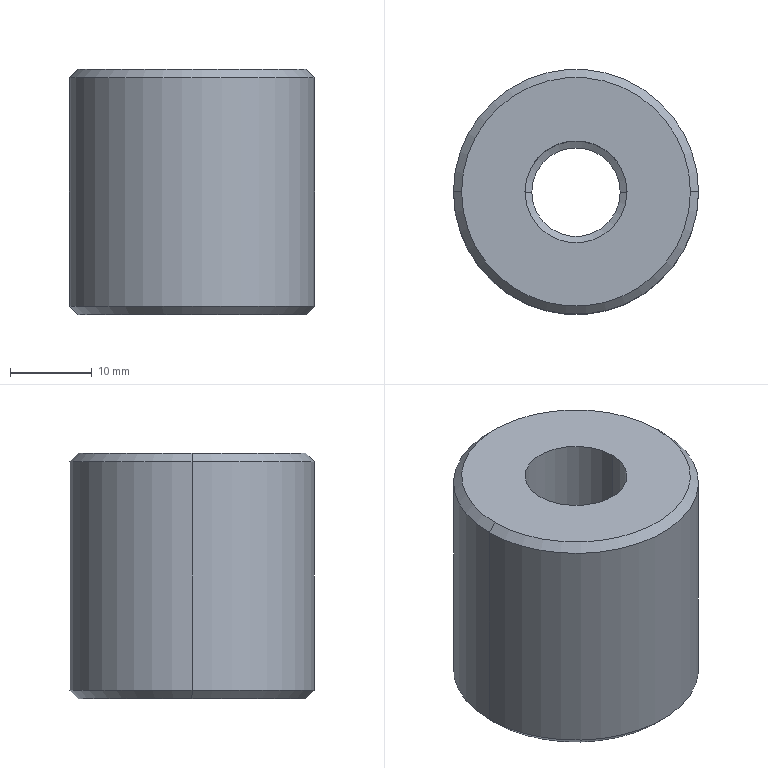Part | STEP file | Locking Cylinder Joint | 1 solid | 15 faces | box 30 x 30 x 30 mm | volume 16100 mm3 | cone 6 | cylinder 6 | plane 3 | commonest cylinder face diameters 12.5 x2 20 x2 30 x2
STEP:
#1=CARTESIAN_POINT('',(0.,0.,0.));
#2=DIRECTION('',(0.,0.,1.));
#3=DIRECTION('',(1.,0.,0.));
#4=AXIS2_PLACEMENT_3D('',#1,#2,#3);
#5=CARTESIAN_POINT('',(-14.,0.,0.));
#6=VERTEX_POINT('',#5);
#7=CARTESIAN_POINT('',(14.,0.,0.));
#8=VERTEX_POINT('',#7);
#9=CARTESIAN_POINT('',(0.,0.,0.));
#10=DIRECTION('',(0.,0.,-1.));
#11=DIRECTION('',(1.,0.,0.));
#12=AXIS2_PLACEMENT_3D('',#9,#10,#11);
#13=CIRCLE('',#12,14.);
#14=CARTESIAN_POINT('',(0.,0.,1.));
#15=DIRECTION('',(0.,0.,1.));
#16=DIRECTION('',(1.,0.,0.));
#17=AXIS2_PLACEMENT_3D('',#14,#15,#16);
#18=CONICAL_SURFACE('',#17,15.,0.7854);
#19=CARTESIAN_POINT('',(6.283,-1.));
#20=DIRECTION('',(-1.,0.));
#21=VECTOR('',#20,1.);
#22=LINE('',#19,#21);
#23=(GEOMETRIC_REPRESENTATION_CONTEXT(2)PARAMETRIC_REPRESENTATION_CONTEXT()REPRESENTATION_CONTEXT('',''));
#24=DEFINITIONAL_REPRESENTATION('',(#22),#23);
#25=PCURVE('',#18,#24);
#26=CARTESIAN_POINT('',(0.,0.,0.));
#27=DIRECTION('',(0.,0.,1.));
#28=DIRECTION('',(1.,0.,0.));
#29=AXIS2_PLACEMENT_3D('',#26,#27,#28);
#30=PLANE('',#29);
#31=CARTESIAN_POINT('',(14.,0.));
#32=CARTESIAN_POINT('',(14.,-24.249));
#33=CARTESIAN_POINT('',(-7.,-12.124));
#34=CARTESIAN_POINT('',(-28.,0.));
#35=CARTESIAN_POINT('',(-7.,12.124));
#36=CARTESIAN_POINT('',(14.,24.249));
#37=CARTESIAN_POINT('',(14.,0.));
#38=(BOUNDED_CURVE()B_SPLINE_CURVE(2,(#31,#32,#33,#34,#35,#36,#37),.UNSPECIFIED.,.T.,.F.)B_SPLINE_CURVE_WITH_KNOTS((1,2,2,2,2,1),(-2.094,0.,2.094,4.189,6.283,8.378),.UNSPECIFIED.)CURVE()GEOMETRIC_REPRESENTATION_ITEM()RATIONAL_B_SPLINE_CURVE((1.,0.5,1.,0.5,1.,0.5,1.))REPRESENTATION_ITEM(''));
#39=(GEOMETRIC_REPRESENTATION_CONTEXT(2)PARAMETRIC_REPRESENTATION_CONTEXT()REPRESENTATION_CONTEXT('',''));
#40=DEFINITIONAL_REPRESENTATION('',(#38),#39);
#41=PCURVE('',#30,#40);
#42=SURFACE_CURVE('',#13,(#25,#41),.PCURVE_S1.);
#43=EDGE_CURVE('',#6,#8,#42,.T.);
#44=ORIENTED_EDGE('',*,*,#43,.F.);
#45=CARTESIAN_POINT('',(-15.,0.,1.));
#46=VERTEX_POINT('',#45);
#47=CARTESIAN_POINT('',(-15.,0.,1.));
#48=DIRECTION('',(-0.7071,0.,0.7071));
#49=VECTOR('',#48,1.);
#50=LINE('',#47,#49);
#51=CARTESIAN_POINT('',(3.142,0.));
#52=DIRECTION('',(0.,1.));
#53=VECTOR('',#52,1.);
#54=LINE('',#51,#53);
#55=(GEOMETRIC_REPRESENTATION_CONTEXT(2)PARAMETRIC_REPRESENTATION_CONTEXT()REPRESENTATION_CONTEXT('',''));
#56=DEFINITIONAL_REPRESENTATION('',(#54),#55);
#57=PCURVE('',#18,#56);
#58=CARTESIAN_POINT('',(0.,0.,1.));
#59=DIRECTION('',(0.,0.,1.));
#60=DIRECTION('',(1.,0.,0.));
#61=AXIS2_PLACEMENT_3D('',#58,#59,#60);
#62=CONICAL_SURFACE('',#61,15.,0.7854);
#63=CARTESIAN_POINT('',(3.142,0.));
#64=DIRECTION('',(0.,1.));
#65=VECTOR('',#64,1.);
#66=LINE('',#63,#65);
#67=(GEOMETRIC_REPRESENTATION_CONTEXT(2)PARAMETRIC_REPRESENTATION_CONTEXT()REPRESENTATION_CONTEXT('',''));
#68=DEFINITIONAL_REPRESENTATION('',(#66),#67);
#69=PCURVE('',#62,#68);
#70=SURFACE_CURVE('',#50,(#57,#69),.PCURVE_S1.);
#71=EDGE_CURVE('',#6,#46,#70,.T.);
#72=ORIENTED_EDGE('',*,*,#71,.T.);
#73=CARTESIAN_POINT('',(15.,0.,1.));
#74=VERTEX_POINT('',#73);
#75=CARTESIAN_POINT('',(0.,0.,1.));
#76=DIRECTION('',(0.,0.,1.));
#77=DIRECTION('',(1.,0.,0.));
#78=AXIS2_PLACEMENT_3D('',#75,#76,#77);
#79=CIRCLE('',#78,15.);
#80=CARTESIAN_POINT('',(0.,0.));
#81=DIRECTION('',(1.,0.));
#82=VECTOR('',#81,1.);
#83=LINE('',#80,#82);
#84=(GEOMETRIC_REPRESENTATION_CONTEXT(2)PARAMETRIC_REPRESENTATION_CONTEXT()REPRESENTATION_CONTEXT('',''));
#85=DEFINITIONAL_REPRESENTATION('',(#83),#84);
#86=PCURVE('',#18,#85);
#87=CARTESIAN_POINT('',(0.,0.,30.));
#88=DIRECTION('',(0.,0.,-1.));
#89=DIRECTION('',(-1.,0.,0.));
#90=AXIS2_PLACEMENT_3D('',#87,#88,#89);
#91=CYLINDRICAL_SURFACE('',#90,15.);
#92=CARTESIAN_POINT('',(3.142,29.));
#93=DIRECTION('',(-1.,0.));
#94=VECTOR('',#93,1.);
#95=LINE('',#92,#94);
#96=(GEOMETRIC_REPRESENTATION_CONTEXT(2)PARAMETRIC_REPRESENTATION_CONTEXT()REPRESENTATION_CONTEXT('',''));
#97=DEFINITIONAL_REPRESENTATION('',(#95),#96);
#98=PCURVE('',#91,#97);
#99=SURFACE_CURVE('',#79,(#86,#98),.PCURVE_S1.);
#100=EDGE_CURVE('',#74,#46,#99,.T.);
#101=ORIENTED_EDGE('',*,*,#100,.F.);
#102=CARTESIAN_POINT('',(15.,0.,1.));
#103=DIRECTION('',(0.7071,0.,0.7071));
#104=VECTOR('',#103,1.);
#105=LINE('',#102,#104);
#106=CARTESIAN_POINT('',(0.,0.));
#107=DIRECTION('',(0.,1.));
#108=VECTOR('',#107,1.);
#109=LINE('',#106,#108);
#110=(GEOMETRIC_REPRESENTATION_CONTEXT(2)PARAMETRIC_REPRESENTATION_CONTEXT()REPRESENTATION_CONTEXT('',''));
#111=DEFINITIONAL_REPRESENTATION('',(#109),#110);
#112=PCURVE('',#18,#111);
#113=CARTESIAN_POINT('',(6.283,0.));
#114=DIRECTION('',(0.,1.));
#115=VECTOR('',#114,1.);
#116=LINE('',#113,#115);
#117=(GEOMETRIC_REPRESENTATION_CONTEXT(2)PARAMETRIC_REPRESENTATION_CONTEXT()REPRESENTATION_CONTEXT('',''));
#118=DEFINITIONAL_REPRESENTATION('',(#116),#117);
#119=PCURVE('',#62,#118);
#120=SURFACE_CURVE('',#105,(#112,#119),.PCURVE_S1.);
#121=EDGE_CURVE('',#8,#74,#120,.T.);
#122=ORIENTED_EDGE('',*,*,#121,.F.);
#123=EDGE_LOOP('',(#44,#72,#101,#122));
#124=FACE_BOUND('',#123,.T.);
#125=ADVANCED_FACE('',(#124),#18,.T.);
#126=CARTESIAN_POINT('',(14.,0.,30.));
#127=VERTEX_POINT('',#126);
#128=CARTESIAN_POINT('',(-14.,0.,30.));
#129=VERTEX_POINT('',#128);
#130=CARTESIAN_POINT('',(0.,0.,30.));
#131=DIRECTION('',(0.,0.,1.));
#132=DIRECTION('',(1.,0.,0.));
#133=AXIS2_PLACEMENT_3D('',#130,#131,#132);
#134=CIRCLE('',#133,14.);
#135=CARTESIAN_POINT('',(0.,0.,30.));
#136=DIRECTION('',(0.,0.,-1.));
#137=DIRECTION('',(-1.,0.,0.));
#138=AXIS2_PLACEMENT_3D('',#135,#136,#137);
#139=CONICAL_SURFACE('',#138,14.,0.7854);
#140=CARTESIAN_POINT('',(3.142,0.));
#141=DIRECTION('',(-1.,0.));
#142=VECTOR('',#141,1.);
#143=LINE('',#140,#142);
#144=(GEOMETRIC_REPRESENTATION_CONTEXT(2)PARAMETRIC_REPRESENTATION_CONTEXT()REPRESENTATION_CONTEXT('',''));
#145=DEFINITIONAL_REPRESENTATION('',(#143),#144);
#146=PCURVE('',#139,#145);
#147=CARTESIAN_POINT('',(0.,0.,30.));
#148=DIRECTION('',(0.,0.,1.));
#149=DIRECTION('',(1.,0.,0.));
#150=AXIS2_PLACEMENT_3D('',#147,#148,#149);
#151=PLANE('',#150);
#152=CARTESIAN_POINT('',(0.,0.));
#153=DIRECTION('',(1.,0.));
#154=AXIS2_PLACEMENT_2D('',#152,#153);
#155=CIRCLE('',#154,14.);
#156=(GEOMETRIC_REPRESENTATION_CONTEXT(2)PARAMETRIC_REPRESENTATION_CONTEXT()REPRESENTATION_CONTEXT('',''));
#157=DEFINITIONAL_REPRESENTATION('',(#155),#156);
#158=PCURVE('',#151,#157);
#159=SURFACE_CURVE('',#134,(#146,#158),.PCURVE_S1.);
#160=EDGE_CURVE('',#127,#129,#159,.T.);
#161=ORIENTED_EDGE('',*,*,#160,.F.);
#162=CARTESIAN_POINT('',(15.,0.,29.));
#163=VERTEX_POINT('',#162);
#164=CARTESIAN_POINT('',(14.,0.,30.));
#165=DIRECTION('',(0.7071,0.,-0.7071));
#166=VECTOR('',#165,1.);
#167=LINE('',#164,#166);
#168=CARTESIAN_POINT('',(3.142,0.));
#169=DIRECTION('',(0.,1.));
#170=VECTOR('',#169,1.);
#171=LINE('',#168,#170);
#172=(GEOMETRIC_REPRESENTATION_CONTEXT(2)PARAMETRIC_REPRESENTATION_CONTEXT()REPRESENTATION_CONTEXT('',''));
#173=DEFINITIONAL_REPRESENTATION('',(#171),#172);
#174=PCURVE('',#139,#173);
#175=CARTESIAN_POINT('',(0.,0.,30.));
#176=DIRECTION('',(0.,0.,-1.));
#177=DIRECTION('',(-1.,0.,0.));
#178=AXIS2_PLACEMENT_3D('',#175,#176,#177);
#179=CONICAL_SURFACE('',#178,14.,0.7854);
#180=CARTESIAN_POINT('',(3.142,0.));
#181=DIRECTION('',(0.,1.));
#182=VECTOR('',#181,1.);
#183=LINE('',#180,#182);
#184=(GEOMETRIC_REPRESENTATION_CONTEXT(2)PARAMETRIC_REPRESENTATION_CONTEXT()REPRESENTATION_CONTEXT('',''));
#185=DEFINITIONAL_REPRESENTATION('',(#183),#184);
#186=PCURVE('',#179,#185);
#187=SURFACE_CURVE('',#167,(#174,#186),.PCURVE_S1.);
#188=EDGE_CURVE('',#127,#163,#187,.T.);
#189=ORIENTED_EDGE('',*,*,#188,.T.);
#190=CARTESIAN_POINT('',(-15.,0.,29.));
#191=VERTEX_POINT('',#190);
#192=CARTESIAN_POINT('',(0.,0.,29.));
#193=DIRECTION('',(0.,0.,-1.));
#194=DIRECTION('',(1.,0.,0.));
#195=AXIS2_PLACEMENT_3D('',#192,#193,#194);
#196=CIRCLE('',#195,15.);
#197=CARTESIAN_POINT('',(-3.142,1.));
#198=DIRECTION('',(1.,0.));
#199=VECTOR('',#198,1.);
#200=LINE('',#197,#199);
#201=(GEOMETRIC_REPRESENTATION_CONTEXT(2)PARAMETRIC_REPRESENTATION_CONTEXT()REPRESENTATION_CONTEXT('',''));
#202=DEFINITIONAL_REPRESENTATION('',(#200),#201);
#203=PCURVE('',#139,#202);
#204=CARTESIAN_POINT('',(-3.142,1.));
#205=DIRECTION('',(1.,0.));
#206=VECTOR('',#205,1.);
#207=LINE('',#204,#206);
#208=(GEOMETRIC_REPRESENTATION_CONTEXT(2)PARAMETRIC_REPRESENTATION_CONTEXT()REPRESENTATION_CONTEXT('',''));
#209=DEFINITIONAL_REPRESENTATION('',(#207),#208);
#210=PCURVE('',#91,#209);
#211=SURFACE_CURVE('',#196,(#203,#210),.PCURVE_S1.);
#212=EDGE_CURVE('',#191,#163,#211,.T.);
#213=ORIENTED_EDGE('',*,*,#212,.F.);
#214=CARTESIAN_POINT('',(-14.,0.,30.));
#215=DIRECTION('',(-0.7071,0.,-0.7071));
#216=VECTOR('',#215,1.);
#217=LINE('',#214,#216);
#218=CARTESIAN_POINT('',(0.,0.));
#219=DIRECTION('',(0.,1.));
#220=VECTOR('',#219,1.);
#221=LINE('',#218,#220);
#222=(GEOMETRIC_REPRESENTATION_CONTEXT(2)PARAMETRIC_REPRESENTATION_CONTEXT()REPRESENTATION_CONTEXT('',''));
#223=DEFINITIONAL_REPRESENTATION('',(#221),#222);
#224=PCURVE('',#139,#223);
#225=CARTESIAN_POINT('',(6.283,0.));
#226=DIRECTION('',(0.,1.));
#227=VECTOR('',#226,1.);
#228=LINE('',#225,#227);
#229=(GEOMETRIC_REPRESENTATION_CONTEXT(2)PARAMETRIC_REPRESENTATION_CONTEXT()REPRESENTATION_CONTEXT('',''));
#230=DEFINITIONAL_REPRESENTATION('',(#228),#229);
#231=PCURVE('',#179,#230);
#232=SURFACE_CURVE('',#217,(#224,#231),.PCURVE_S1.);
#233=EDGE_CURVE('',#129,#191,#232,.T.);
#234=ORIENTED_EDGE('',*,*,#233,.F.);
#235=EDGE_LOOP('',(#161,#189,#213,#234));
#236=FACE_BOUND('',#235,.T.);
#237=ADVANCED_FACE('',(#236),#139,.T.);
#238=CARTESIAN_POINT('',(-10.,0.,7.));
#239=VERTEX_POINT('',#238);
#240=CARTESIAN_POINT('',(-10.,0.,0.));
#241=VERTEX_POINT('',#240);
#242=CARTESIAN_POINT('',(-10.,0.,7.));
#243=DIRECTION('',(0.,0.,-1.));
#244=VECTOR('',#243,1.);
#245=LINE('',#242,#244);
#246=CARTESIAN_POINT('',(0.,0.,7.));
#247=DIRECTION('',(0.,0.,-1.));
#248=DIRECTION('',(-1.,0.,0.));
#249=AXIS2_PLACEMENT_3D('',#246,#247,#248);
#250=CYLINDRICAL_SURFACE('',#249,10.);
#251=CARTESIAN_POINT('',(6.283,0.));
#252=DIRECTION('',(0.,1.));
#253=VECTOR('',#252,1.);
#254=LINE('',#251,#253);
#255=(GEOMETRIC_REPRESENTATION_CONTEXT(2)PARAMETRIC_REPRESENTATION_CONTEXT()REPRESENTATION_CONTEXT('',''));
#256=DEFINITIONAL_REPRESENTATION('',(#254),#255);
#257=PCURVE('',#250,#256);
#258=CARTESIAN_POINT('',(0.,0.,7.));
#259=DIRECTION('',(0.,0.,-1.));
#260=DIRECTION('',(-1.,0.,0.));
#261=AXIS2_PLACEMENT_3D('',#258,#259,#260);
#262=CYLINDRICAL_SURFACE('',#261,10.);
#263=CARTESIAN_POINT('',(0.,0.));
#264=DIRECTION('',(0.,1.));
#265=VECTOR('',#264,1.);
#266=LINE('',#263,#265);
#267=(GEOMETRIC_REPRESENTATION_CONTEXT(2)PARAMETRIC_REPRESENTATION_CONTEXT()REPRESENTATION_CONTEXT('',''));
#268=DEFINITIONAL_REPRESENTATION('',(#266),#267);
#269=PCURVE('',#262,#268);
#270=SURFACE_CURVE('',#245,(#257,#269),.PCURVE_S1.);
#271=EDGE_CURVE('',#239,#241,#270,.T.);
#272=ORIENTED_EDGE('',*,*,#271,.T.);
#273=CARTESIAN_POINT('',(10.,0.,0.));
#274=VERTEX_POINT('',#273);
#275=CARTESIAN_POINT('',(0.,0.,0.));
#276=DIRECTION('',(0.,0.,-1.));
#277=DIRECTION('',(-1.,0.,0.));
#278=AXIS2_PLACEMENT_3D('',#275,#276,#277);
#279=CIRCLE('',#278,10.);
#280=CARTESIAN_POINT('',(0.,7.));
#281=DIRECTION('',(1.,0.));
#282=VECTOR('',#281,1.);
#283=LINE('',#280,#282);
#284=(GEOMETRIC_REPRESENTATION_CONTEXT(2)PARAMETRIC_REPRESENTATION_CONTEXT()REPRESENTATION_CONTEXT('',''));
#285=DEFINITIONAL_REPRESENTATION('',(#283),#284);
#286=PCURVE('',#250,#285);
#287=CARTESIAN_POINT('',(-10.,0.));
#288=CARTESIAN_POINT('',(-10.,17.321));
#289=CARTESIAN_POINT('',(5.,8.66));
#290=CARTESIAN_POINT('',(20.,0.));
#291=CARTESIAN_POINT('',(5.,-8.66));
#292=CARTESIAN_POINT('',(-10.,-17.321));
#293=CARTESIAN_POINT('',(-10.,0.));
#294=(BOUNDED_CURVE()B_SPLINE_CURVE(2,(#287,#288,#289,#290,#291,#292,#293),.UNSPECIFIED.,.T.,.F.)B_SPLINE_CURVE_WITH_KNOTS((1,2,2,2,2,1),(-2.094,0.,2.094,4.189,6.283,8.378),.UNSPECIFIED.)CURVE()GEOMETRIC_REPRESENTATION_ITEM()RATIONAL_B_SPLINE_CURVE((1.,0.5,1.,0.5,1.,0.5,1.))REPRESENTATION_ITEM(''));
#295=(GEOMETRIC_REPRESENTATION_CONTEXT(2)PARAMETRIC_REPRESENTATION_CONTEXT()REPRESENTATION_CONTEXT('',''));
#296=DEFINITIONAL_REPRESENTATION('',(#294),#295);
#297=PCURVE('',#30,#296);
#298=SURFACE_CURVE('',#279,(#286,#297),.PCURVE_S1.);
#299=EDGE_CURVE('',#274,#241,#298,.T.);
#300=ORIENTED_EDGE('',*,*,#299,.F.);
#301=CARTESIAN_POINT('',(10.,0.,7.));
#302=VERTEX_POINT('',#301);
#303=CARTESIAN_POINT('',(10.,0.,7.));
#304=DIRECTION('',(0.,0.,-1.));
#305=VECTOR('',#304,1.);
#306=LINE('',#303,#305);
#307=CARTESIAN_POINT('',(3.142,0.));
#308=DIRECTION('',(0.,1.));
#309=VECTOR('',#308,1.);
#310=LINE('',#307,#309);
#311=(GEOMETRIC_REPRESENTATION_CONTEXT(2)PARAMETRIC_REPRESENTATION_CONTEXT()REPRESENTATION_CONTEXT('',''));
#312=DEFINITIONAL_REPRESENTATION('',(#310),#311);
#313=PCURVE('',#250,#312);
#314=CARTESIAN_POINT('',(3.142,0.));
#315=DIRECTION('',(0.,1.));
#316=VECTOR('',#315,1.);
#317=LINE('',#314,#316);
#318=(GEOMETRIC_REPRESENTATION_CONTEXT(2)PARAMETRIC_REPRESENTATION_CONTEXT()REPRESENTATION_CONTEXT('',''));
#319=DEFINITIONAL_REPRESENTATION('',(#317),#318);
#320=PCURVE('',#262,#319);
#321=SURFACE_CURVE('',#306,(#313,#320),.PCURVE_S1.);
#322=EDGE_CURVE('',#302,#274,#321,.T.);
#323=ORIENTED_EDGE('',*,*,#322,.F.);
#324=CARTESIAN_POINT('',(0.,0.,7.));
#325=DIRECTION('',(0.,0.,-1.));
#326=DIRECTION('',(-1.,0.,0.));
#327=AXIS2_PLACEMENT_3D('',#324,#325,#326);
#328=CIRCLE('',#327,10.);
#329=CARTESIAN_POINT('',(0.,0.));
#330=DIRECTION('',(1.,0.));
#331=VECTOR('',#330,1.);
#332=LINE('',#329,#331);
#333=(GEOMETRIC_REPRESENTATION_CONTEXT(2)PARAMETRIC_REPRESENTATION_CONTEXT()REPRESENTATION_CONTEXT('',''));
#334=DEFINITIONAL_REPRESENTATION('',(#332),#333);
#335=PCURVE('',#250,#334);
#336=CARTESIAN_POINT('',(0.,0.,7.));
#337=DIRECTION('',(0.,0.,-1.));
#338=DIRECTION('',(-1.,0.,0.));
#339=AXIS2_PLACEMENT_3D('',#336,#337,#338);
#340=PLANE('',#339);
#341=CARTESIAN_POINT('',(0.,0.));
#342=DIRECTION('',(1.,0.));
#343=AXIS2_PLACEMENT_2D('',#341,#342);
#344=CIRCLE('',#343,10.);
#345=(GEOMETRIC_REPRESENTATION_CONTEXT(2)PARAMETRIC_REPRESENTATION_CONTEXT()REPRESENTATION_CONTEXT('',''));
#346=DEFINITIONAL_REPRESENTATION('',(#344),#345);
#347=PCURVE('',#340,#346);
#348=SURFACE_CURVE('',#328,(#335,#347),.PCURVE_S1.);
#349=EDGE_CURVE('',#302,#239,#348,.T.);
#350=ORIENTED_EDGE('',*,*,#349,.T.);
#351=EDGE_LOOP('',(#272,#300,#323,#350));
#352=FACE_BOUND('',#351,.F.);
#353=ADVANCED_FACE('',(#352),#250,.F.);
#354=CARTESIAN_POINT('',(6.25,0.,7.5));
#355=VERTEX_POINT('',#354);
#356=CARTESIAN_POINT('',(6.25,0.,30.));
#357=VERTEX_POINT('',#356);
#358=CARTESIAN_POINT('',(6.25,0.,30.));
#359=DIRECTION('',(0.,0.,1.));
#360=VECTOR('',#359,1.);
#361=LINE('',#358,#360);
#362=CARTESIAN_POINT('',(0.,0.,30.));
#363=DIRECTION('',(0.,0.,1.));
#364=DIRECTION('',(1.,0.,0.));
#365=AXIS2_PLACEMENT_3D('',#362,#363,#364);
#366=CYLINDRICAL_SURFACE('',#365,6.25);
#367=CARTESIAN_POINT('',(6.283,0.));
#368=DIRECTION('',(0.,1.));
#369=VECTOR('',#368,1.);
#370=LINE('',#367,#369);
#371=(GEOMETRIC_REPRESENTATION_CONTEXT(2)PARAMETRIC_REPRESENTATION_CONTEXT()REPRESENTATION_CONTEXT('',''));
#372=DEFINITIONAL_REPRESENTATION('',(#370),#371);
#373=PCURVE('',#366,#372);
#374=CARTESIAN_POINT('',(0.,0.,30.));
#375=DIRECTION('',(0.,0.,1.));
#376=DIRECTION('',(1.,0.,0.));
#377=AXIS2_PLACEMENT_3D('',#374,#375,#376);
#378=CYLINDRICAL_SURFACE('',#377,6.25);
#379=CARTESIAN_POINT('',(0.,0.));
#380=DIRECTION('',(0.,1.));
#381=VECTOR('',#380,1.);
#382=LINE('',#379,#381);
#383=(GEOMETRIC_REPRESENTATION_CONTEXT(2)PARAMETRIC_REPRESENTATION_CONTEXT()REPRESENTATION_CONTEXT('',''));
#384=DEFINITIONAL_REPRESENTATION('',(#382),#383);
#385=PCURVE('',#378,#384);
#386=SURFACE_CURVE('',#361,(#373,#385),.PCURVE_S1.);
#387=EDGE_CURVE('',#355,#357,#386,.T.);
#388=ORIENTED_EDGE('',*,*,#387,.T.);
#389=CARTESIAN_POINT('',(-6.25,0.,30.));
#390=VERTEX_POINT('',#389);
#391=CARTESIAN_POINT('',(0.,0.,30.));
#392=DIRECTION('',(0.,0.,1.));
#393=DIRECTION('',(1.,0.,0.));
#394=AXIS2_PLACEMENT_3D('',#391,#392,#393);
#395=CIRCLE('',#394,6.25);
#396=CARTESIAN_POINT('',(0.,0.));
#397=DIRECTION('',(1.,0.));
#398=VECTOR('',#397,1.);
#399=LINE('',#396,#398);
#400=(GEOMETRIC_REPRESENTATION_CONTEXT(2)PARAMETRIC_REPRESENTATION_CONTEXT()REPRESENTATION_CONTEXT('',''));
#401=DEFINITIONAL_REPRESENTATION('',(#399),#400);
#402=PCURVE('',#366,#401);
#403=CARTESIAN_POINT('',(0.,0.));
#404=DIRECTION('',(1.,0.));
#405=AXIS2_PLACEMENT_2D('',#403,#404);
#406=CIRCLE('',#405,6.25);
#407=(GEOMETRIC_REPRESENTATION_CONTEXT(2)PARAMETRIC_REPRESENTATION_CONTEXT()REPRESENTATION_CONTEXT('',''));
#408=DEFINITIONAL_REPRESENTATION('',(#406),#407);
#409=PCURVE('',#151,#408);
#410=SURFACE_CURVE('',#395,(#402,#409),.PCURVE_S1.);
#411=EDGE_CURVE('',#390,#357,#410,.T.);
#412=ORIENTED_EDGE('',*,*,#411,.F.);
#413=CARTESIAN_POINT('',(-6.25,0.,7.5));
#414=VERTEX_POINT('',#413);
#415=CARTESIAN_POINT('',(-6.25,0.,30.));
#416=DIRECTION('',(0.,0.,1.));
#417=VECTOR('',#416,1.);
#418=LINE('',#415,#417);
#419=CARTESIAN_POINT('',(3.142,0.));
#420=DIRECTION('',(0.,1.));
#421=VECTOR('',#420,1.);
#422=LINE('',#419,#421);
#423=(GEOMETRIC_REPRESENTATION_CONTEXT(2)PARAMETRIC_REPRESENTATION_CONTEXT()REPRESENTATION_CONTEXT('',''));
#424=DEFINITIONAL_REPRESENTATION('',(#422),#423);
#425=PCURVE('',#366,#424);
#426=CARTESIAN_POINT('',(3.142,0.));
#427=DIRECTION('',(0.,1.));
#428=VECTOR('',#427,1.);
#429=LINE('',#426,#428);
#430=(GEOMETRIC_REPRESENTATION_CONTEXT(2)PARAMETRIC_REPRESENTATION_CONTEXT()REPRESENTATION_CONTEXT('',''));
#431=DEFINITIONAL_REPRESENTATION('',(#429),#430);
#432=PCURVE('',#378,#431);
#433=SURFACE_CURVE('',#418,(#425,#432),.PCURVE_S1.);
#434=EDGE_CURVE('',#414,#390,#433,.T.);
#435=ORIENTED_EDGE('',*,*,#434,.F.);
#436=CARTESIAN_POINT('',(0.,0.,7.5));
#437=DIRECTION('',(0.,0.,1.));
#438=DIRECTION('',(1.,0.,0.));
#439=AXIS2_PLACEMENT_3D('',#436,#437,#438);
#440=CIRCLE('',#439,6.25);
#441=CARTESIAN_POINT('',(0.,-22.5));
#442=DIRECTION('',(1.,0.));
#443=VECTOR('',#442,1.);
#444=LINE('',#441,#443);
#445=(GEOMETRIC_REPRESENTATION_CONTEXT(2)PARAMETRIC_REPRESENTATION_CONTEXT()REPRESENTATION_CONTEXT('',''));
#446=DEFINITIONAL_REPRESENTATION('',(#444),#445);
#447=PCURVE('',#366,#446);
#448=CARTESIAN_POINT('',(0.,0.,7.5));
#449=DIRECTION('',(0.,0.,1.));
#450=DIRECTION('',(1.,0.,0.));
#451=AXIS2_PLACEMENT_3D('',#448,#449,#450);
#452=CONICAL_SURFACE('',#451,6.25,1.03);
#453=CARTESIAN_POINT('',(0.,0.));
#454=DIRECTION('',(1.,0.));
#455=VECTOR('',#454,1.);
#456=LINE('',#453,#455);
#457=(GEOMETRIC_REPRESENTATION_CONTEXT(2)PARAMETRIC_REPRESENTATION_CONTEXT()REPRESENTATION_CONTEXT('',''));
#458=DEFINITIONAL_REPRESENTATION('',(#456),#457);
#459=PCURVE('',#452,#458);
#460=SURFACE_CURVE('',#440,(#447,#459),.PCURVE_S1.);
#461=EDGE_CURVE('',#414,#355,#460,.T.);
#462=ORIENTED_EDGE('',*,*,#461,.T.);
#463=EDGE_LOOP('',(#388,#412,#435,#462));
#464=FACE_BOUND('',#463,.F.);
#465=ADVANCED_FACE('',(#464),#366,.F.);
#466=ORIENTED_EDGE('',*,*,#212,.T.);
#467=CARTESIAN_POINT('',(15.,0.,30.));
#468=DIRECTION('',(0.,0.,-1.));
#469=VECTOR('',#468,1.);
#470=LINE('',#467,#469);
#471=CARTESIAN_POINT('',(3.142,0.));
#472=DIRECTION('',(0.,1.));
#473=VECTOR('',#472,1.);
#474=LINE('',#471,#473);
#475=(GEOMETRIC_REPRESENTATION_CONTEXT(2)PARAMETRIC_REPRESENTATION_CONTEXT()REPRESENTATION_CONTEXT('',''));
#476=DEFINITIONAL_REPRESENTATION('',(#474),#475);
#477=PCURVE('',#91,#476);
#478=CARTESIAN_POINT('',(0.,0.,30.));
#479=DIRECTION('',(0.,0.,-1.));
#480=DIRECTION('',(-1.,0.,0.));
#481=AXIS2_PLACEMENT_3D('',#478,#479,#480);
#482=CYLINDRICAL_SURFACE('',#481,15.);
#483=CARTESIAN_POINT('',(3.142,0.));
#484=DIRECTION('',(0.,1.));
#485=VECTOR('',#484,1.);
#486=LINE('',#483,#485);
#487=(GEOMETRIC_REPRESENTATION_CONTEXT(2)PARAMETRIC_REPRESENTATION_CONTEXT()REPRESENTATION_CONTEXT('',''));
#488=DEFINITIONAL_REPRESENTATION('',(#486),#487);
#489=PCURVE('',#482,#488);
#490=SURFACE_CURVE('',#470,(#477,#489),.PCURVE_S1.);
#491=EDGE_CURVE('',#163,#74,#490,.T.);
#492=ORIENTED_EDGE('',*,*,#491,.T.);
#493=ORIENTED_EDGE('',*,*,#100,.T.);
#494=CARTESIAN_POINT('',(-15.,0.,30.));
#495=DIRECTION('',(0.,0.,-1.));
#496=VECTOR('',#495,1.);
#497=LINE('',#494,#496);
#498=CARTESIAN_POINT('',(0.,0.));
#499=DIRECTION('',(0.,1.));
#500=VECTOR('',#499,1.);
#501=LINE('',#498,#500);
#502=(GEOMETRIC_REPRESENTATION_CONTEXT(2)PARAMETRIC_REPRESENTATION_CONTEXT()REPRESENTATION_CONTEXT('',''));
#503=DEFINITIONAL_REPRESENTATION('',(#501),#502);
#504=PCURVE('',#91,#503);
#505=CARTESIAN_POINT('',(6.283,0.));
#506=DIRECTION('',(0.,1.));
#507=VECTOR('',#506,1.);
#508=LINE('',#505,#507);
#509=(GEOMETRIC_REPRESENTATION_CONTEXT(2)PARAMETRIC_REPRESENTATION_CONTEXT()REPRESENTATION_CONTEXT('',''));
#510=DEFINITIONAL_REPRESENTATION('',(#508),#509);
#511=PCURVE('',#482,#510);
#512=SURFACE_CURVE('',#497,(#504,#511),.PCURVE_S1.);
#513=EDGE_CURVE('',#191,#46,#512,.T.);
#514=ORIENTED_EDGE('',*,*,#513,.F.);
#515=EDGE_LOOP('',(#466,#492,#493,#514));
#516=FACE_BOUND('',#515,.T.);
#517=ADVANCED_FACE('',(#516),#91,.T.);
#518=CARTESIAN_POINT('',(5.418,0.,7.));
#519=VERTEX_POINT('',#518);
#520=CARTESIAN_POINT('',(6.25,0.,7.5));
#521=DIRECTION('',(0.8572,0.,0.515));
#522=VECTOR('',#521,1.);
#523=LINE('',#520,#522);
#524=CARTESIAN_POINT('',(6.283,0.));
#525=DIRECTION('',(0.,1.));
#526=VECTOR('',#525,1.);
#527=LINE('',#524,#526);
#528=(GEOMETRIC_REPRESENTATION_CONTEXT(2)PARAMETRIC_REPRESENTATION_CONTEXT()REPRESENTATION_CONTEXT('',''));
#529=DEFINITIONAL_REPRESENTATION('',(#527),#528);
#530=PCURVE('',#452,#529);
#531=CARTESIAN_POINT('',(0.,0.,7.5));
#532=DIRECTION('',(0.,0.,1.));
#533=DIRECTION('',(1.,0.,0.));
#534=AXIS2_PLACEMENT_3D('',#531,#532,#533);
#535=CONICAL_SURFACE('',#534,6.25,1.03);
#536=CARTESIAN_POINT('',(0.,0.));
#537=DIRECTION('',(0.,1.));
#538=VECTOR('',#537,1.);
#539=LINE('',#536,#538);
#540=(GEOMETRIC_REPRESENTATION_CONTEXT(2)PARAMETRIC_REPRESENTATION_CONTEXT()REPRESENTATION_CONTEXT('',''));
#541=DEFINITIONAL_REPRESENTATION('',(#539),#540);
#542=PCURVE('',#535,#541);
#543=SURFACE_CURVE('',#523,(#530,#542),.PCURVE_S1.);
#544=EDGE_CURVE('',#519,#355,#543,.T.);
#545=ORIENTED_EDGE('',*,*,#544,.T.);
#546=ORIENTED_EDGE('',*,*,#461,.F.);
#547=CARTESIAN_POINT('',(-5.418,0.,7.));
#548=VERTEX_POINT('',#547);
#549=CARTESIAN_POINT('',(-6.25,0.,7.5));
#550=DIRECTION('',(-0.8572,0.,0.515));
#551=VECTOR('',#550,1.);
#552=LINE('',#549,#551);
#553=CARTESIAN_POINT('',(3.142,0.));
#554=DIRECTION('',(0.,1.));
#555=VECTOR('',#554,1.);
#556=LINE('',#553,#555);
#557=(GEOMETRIC_REPRESENTATION_CONTEXT(2)PARAMETRIC_REPRESENTATION_CONTEXT()REPRESENTATION_CONTEXT('',''));
#558=DEFINITIONAL_REPRESENTATION('',(#556),#557);
#559=PCURVE('',#452,#558);
#560=CARTESIAN_POINT('',(3.142,0.));
#561=DIRECTION('',(0.,1.));
#562=VECTOR('',#561,1.);
#563=LINE('',#560,#562);
#564=(GEOMETRIC_REPRESENTATION_CONTEXT(2)PARAMETRIC_REPRESENTATION_CONTEXT()REPRESENTATION_CONTEXT('',''));
#565=DEFINITIONAL_REPRESENTATION('',(#563),#564);
#566=PCURVE('',#535,#565);
#567=SURFACE_CURVE('',#552,(#559,#566),.PCURVE_S1.);
#568=EDGE_CURVE('',#548,#414,#567,.T.);
#569=ORIENTED_EDGE('',*,*,#568,.F.);
#570=CARTESIAN_POINT('',(0.,0.,7.));
#571=DIRECTION('',(0.,0.,1.));
#572=DIRECTION('',(-1.,0.,0.));
#573=AXIS2_PLACEMENT_3D('',#570,#571,#572);
#574=CIRCLE('',#573,5.418);
#575=CARTESIAN_POINT('',(3.142,-0.5));
#576=DIRECTION('',(1.,0.));
#577=VECTOR('',#576,1.);
#578=LINE('',#575,#577);
#579=(GEOMETRIC_REPRESENTATION_CONTEXT(2)PARAMETRIC_REPRESENTATION_CONTEXT()REPRESENTATION_CONTEXT('',''));
#580=DEFINITIONAL_REPRESENTATION('',(#578),#579);
#581=PCURVE('',#452,#580);
#582=CARTESIAN_POINT('',(5.418,0.));
#583=CARTESIAN_POINT('',(5.418,-9.384));
#584=CARTESIAN_POINT('',(-2.709,-4.692));
#585=CARTESIAN_POINT('',(-10.836,0.));
#586=CARTESIAN_POINT('',(-2.709,4.692));
#587=CARTESIAN_POINT('',(5.418,9.384));
#588=CARTESIAN_POINT('',(5.418,0.));
#589=(BOUNDED_CURVE()B_SPLINE_CURVE(2,(#582,#583,#584,#585,#586,#587,#588),.UNSPECIFIED.,.T.,.F.)B_SPLINE_CURVE_WITH_KNOTS((1,2,2,2,2,1),(-2.094,0.,2.094,4.189,6.283,8.378),.UNSPECIFIED.)CURVE()GEOMETRIC_REPRESENTATION_ITEM()RATIONAL_B_SPLINE_CURVE((1.,0.5,1.,0.5,1.,0.5,1.))REPRESENTATION_ITEM(''));
#590=(GEOMETRIC_REPRESENTATION_CONTEXT(2)PARAMETRIC_REPRESENTATION_CONTEXT()REPRESENTATION_CONTEXT('',''));
#591=DEFINITIONAL_REPRESENTATION('',(#589),#590);
#592=PCURVE('',#340,#591);
#593=SURFACE_CURVE('',#574,(#581,#592),.PCURVE_S1.);
#594=EDGE_CURVE('',#548,#519,#593,.T.);
#595=ORIENTED_EDGE('',*,*,#594,.T.);
#596=EDGE_LOOP('',(#545,#546,#569,#595));
#597=FACE_BOUND('',#596,.F.);
#598=ADVANCED_FACE('',(#597),#452,.F.);
#599=CARTESIAN_POINT('',(0.,0.,7.5));
#600=DIRECTION('',(0.,0.,1.));
#601=DIRECTION('',(1.,0.,0.));
#602=AXIS2_PLACEMENT_3D('',#599,#600,#601);
#603=CIRCLE('',#602,6.25);
#604=CARTESIAN_POINT('',(0.,0.));
#605=DIRECTION('',(1.,0.));
#606=VECTOR('',#605,1.);
#607=LINE('',#604,#606);
#608=(GEOMETRIC_REPRESENTATION_CONTEXT(2)PARAMETRIC_REPRESENTATION_CONTEXT()REPRESENTATION_CONTEXT('',''));
#609=DEFINITIONAL_REPRESENTATION('',(#607),#608);
#610=PCURVE('',#535,#609);
#611=CARTESIAN_POINT('',(0.,-22.5));
#612=DIRECTION('',(1.,0.));
#613=VECTOR('',#612,1.);
#614=LINE('',#611,#613);
#615=(GEOMETRIC_REPRESENTATION_CONTEXT(2)PARAMETRIC_REPRESENTATION_CONTEXT()REPRESENTATION_CONTEXT('',''));
#616=DEFINITIONAL_REPRESENTATION('',(#614),#615);
#617=PCURVE('',#378,#616);
#618=SURFACE_CURVE('',#603,(#610,#617),.PCURVE_S1.);
#619=EDGE_CURVE('',#355,#414,#618,.T.);
#620=ORIENTED_EDGE('',*,*,#619,.F.);
#621=ORIENTED_EDGE('',*,*,#544,.F.);
#622=CARTESIAN_POINT('',(0.,0.,7.));
#623=DIRECTION('',(0.,0.,1.));
#624=DIRECTION('',(-1.,0.,0.));
#625=AXIS2_PLACEMENT_3D('',#622,#623,#624);
#626=CIRCLE('',#625,5.418);
#627=CARTESIAN_POINT('',(-3.142,-0.5));
#628=DIRECTION('',(1.,0.));
#629=VECTOR('',#628,1.);
#630=LINE('',#627,#629);
#631=(GEOMETRIC_REPRESENTATION_CONTEXT(2)PARAMETRIC_REPRESENTATION_CONTEXT()REPRESENTATION_CONTEXT('',''));
#632=DEFINITIONAL_REPRESENTATION('',(#630),#631);
#633=PCURVE('',#535,#632);
#634=CARTESIAN_POINT('',(5.418,0.));
#635=CARTESIAN_POINT('',(5.418,-9.384));
#636=CARTESIAN_POINT('',(-2.709,-4.692));
#637=CARTESIAN_POINT('',(-10.836,0.));
#638=CARTESIAN_POINT('',(-2.709,4.692));
#639=CARTESIAN_POINT('',(5.418,9.384));
#640=CARTESIAN_POINT('',(5.418,0.));
#641=(BOUNDED_CURVE()B_SPLINE_CURVE(2,(#634,#635,#636,#637,#638,#639,#640),.UNSPECIFIED.,.T.,.F.)B_SPLINE_CURVE_WITH_KNOTS((1,2,2,2,2,1),(-2.094,0.,2.094,4.189,6.283,8.378),.UNSPECIFIED.)CURVE()GEOMETRIC_REPRESENTATION_ITEM()RATIONAL_B_SPLINE_CURVE((1.,0.5,1.,0.5,1.,0.5,1.))REPRESENTATION_ITEM(''));
#642=(GEOMETRIC_REPRESENTATION_CONTEXT(2)PARAMETRIC_REPRESENTATION_CONTEXT()REPRESENTATION_CONTEXT('',''));
#643=DEFINITIONAL_REPRESENTATION('',(#641),#642);
#644=PCURVE('',#340,#643);
#645=SURFACE_CURVE('',#626,(#633,#644),.PCURVE_S1.);
#646=EDGE_CURVE('',#519,#548,#645,.T.);
#647=ORIENTED_EDGE('',*,*,#646,.T.);
#648=ORIENTED_EDGE('',*,*,#568,.T.);
#649=EDGE_LOOP('',(#620,#621,#647,#648));
#650=FACE_BOUND('',#649,.F.);
#651=ADVANCED_FACE('',(#650),#535,.F.);
#652=ORIENTED_EDGE('',*,*,#491,.F.);
#653=CARTESIAN_POINT('',(0.,0.,29.));
#654=DIRECTION('',(0.,0.,-1.));
#655=DIRECTION('',(1.,0.,0.));
#656=AXIS2_PLACEMENT_3D('',#653,#654,#655);
#657=CIRCLE('',#656,15.);
#658=CARTESIAN_POINT('',(3.142,1.));
#659=DIRECTION('',(1.,0.));
#660=VECTOR('',#659,1.);
#661=LINE('',#658,#660);
#662=(GEOMETRIC_REPRESENTATION_CONTEXT(2)PARAMETRIC_REPRESENTATION_CONTEXT()REPRESENTATION_CONTEXT('',''));
#663=DEFINITIONAL_REPRESENTATION('',(#661),#662);
#664=PCURVE('',#482,#663);
#665=CARTESIAN_POINT('',(3.142,1.));
#666=DIRECTION('',(1.,0.));
#667=VECTOR('',#666,1.);
#668=LINE('',#665,#667);
#669=(GEOMETRIC_REPRESENTATION_CONTEXT(2)PARAMETRIC_REPRESENTATION_CONTEXT()REPRESENTATION_CONTEXT('',''));
#670=DEFINITIONAL_REPRESENTATION('',(#668),#669);
#671=PCURVE('',#179,#670);
#672=SURFACE_CURVE('',#657,(#664,#671),.PCURVE_S1.);
#673=EDGE_CURVE('',#163,#191,#672,.T.);
#674=ORIENTED_EDGE('',*,*,#673,.T.);
#675=ORIENTED_EDGE('',*,*,#513,.T.);
#676=CARTESIAN_POINT('',(0.,0.,1.));
#677=DIRECTION('',(0.,0.,1.));
#678=DIRECTION('',(1.,0.,0.));
#679=AXIS2_PLACEMENT_3D('',#676,#677,#678);
#680=CIRCLE('',#679,15.);
#681=CARTESIAN_POINT('',(9.425,29.));
#682=DIRECTION('',(-1.,0.));
#683=VECTOR('',#682,1.);
#684=LINE('',#681,#683);
#685=(GEOMETRIC_REPRESENTATION_CONTEXT(2)PARAMETRIC_REPRESENTATION_CONTEXT()REPRESENTATION_CONTEXT('',''));
#686=DEFINITIONAL_REPRESENTATION('',(#684),#685);
#687=PCURVE('',#482,#686);
#688=CARTESIAN_POINT('',(0.,0.));
#689=DIRECTION('',(1.,0.));
#690=VECTOR('',#689,1.);
#691=LINE('',#688,#690);
#692=(GEOMETRIC_REPRESENTATION_CONTEXT(2)PARAMETRIC_REPRESENTATION_CONTEXT()REPRESENTATION_CONTEXT('',''));
#693=DEFINITIONAL_REPRESENTATION('',(#691),#692);
#694=PCURVE('',#62,#693);
#695=SURFACE_CURVE('',#680,(#687,#694),.PCURVE_S1.);
#696=EDGE_CURVE('',#46,#74,#695,.T.);
#697=ORIENTED_EDGE('',*,*,#696,.T.);
#698=EDGE_LOOP('',(#652,#674,#675,#697));
#699=FACE_BOUND('',#698,.T.);
#700=ADVANCED_FACE('',(#699),#482,.T.);
#701=CARTESIAN_POINT('',(0.,0.,30.));
#702=DIRECTION('',(0.,0.,1.));
#703=DIRECTION('',(1.,0.,0.));
#704=AXIS2_PLACEMENT_3D('',#701,#702,#703);
#705=CIRCLE('',#704,14.);
#706=CARTESIAN_POINT('',(0.,0.));
#707=DIRECTION('',(1.,0.));
#708=AXIS2_PLACEMENT_2D('',#706,#707);
#709=CIRCLE('',#708,14.);
#710=(GEOMETRIC_REPRESENTATION_CONTEXT(2)PARAMETRIC_REPRESENTATION_CONTEXT()REPRESENTATION_CONTEXT('',''));
#711=DEFINITIONAL_REPRESENTATION('',(#709),#710);
#712=PCURVE('',#151,#711);
#713=CARTESIAN_POINT('',(9.425,0.));
#714=DIRECTION('',(-1.,0.));
#715=VECTOR('',#714,1.);
#716=LINE('',#713,#715);
#717=(GEOMETRIC_REPRESENTATION_CONTEXT(2)PARAMETRIC_REPRESENTATION_CONTEXT()REPRESENTATION_CONTEXT('',''));
#718=DEFINITIONAL_REPRESENTATION('',(#716),#717);
#719=PCURVE('',#179,#718);
#720=SURFACE_CURVE('',#705,(#712,#719),.PCURVE_S1.);
#721=EDGE_CURVE('',#129,#127,#720,.T.);
#722=ORIENTED_EDGE('',*,*,#721,.T.);
#723=ORIENTED_EDGE('',*,*,#160,.T.);
#724=EDGE_LOOP('',(#722,#723));
#725=FACE_BOUND('',#724,.T.);
#726=CARTESIAN_POINT('',(0.,0.,30.));
#727=DIRECTION('',(0.,0.,1.));
#728=DIRECTION('',(1.,0.,0.));
#729=AXIS2_PLACEMENT_3D('',#726,#727,#728);
#730=CIRCLE('',#729,6.25);
#731=CARTESIAN_POINT('',(0.,0.));
#732=DIRECTION('',(1.,0.));
#733=AXIS2_PLACEMENT_2D('',#731,#732);
#734=CIRCLE('',#733,6.25);
#735=(GEOMETRIC_REPRESENTATION_CONTEXT(2)PARAMETRIC_REPRESENTATION_CONTEXT()REPRESENTATION_CONTEXT('',''));
#736=DEFINITIONAL_REPRESENTATION('',(#734),#735);
#737=PCURVE('',#151,#736);
#738=CARTESIAN_POINT('',(0.,0.));
#739=DIRECTION('',(1.,0.));
#740=VECTOR('',#739,1.);
#741=LINE('',#738,#740);
#742=(GEOMETRIC_REPRESENTATION_CONTEXT(2)PARAMETRIC_REPRESENTATION_CONTEXT()REPRESENTATION_CONTEXT('',''));
#743=DEFINITIONAL_REPRESENTATION('',(#741),#742);
#744=PCURVE('',#378,#743);
#745=SURFACE_CURVE('',#730,(#737,#744),.PCURVE_S1.);
#746=EDGE_CURVE('',#357,#390,#745,.T.);
#747=ORIENTED_EDGE('',*,*,#746,.F.);
#748=ORIENTED_EDGE('',*,*,#411,.F.);
#749=EDGE_LOOP('',(#747,#748));
#750=FACE_BOUND('',#749,.T.);
#751=ADVANCED_FACE('',(#725,#750),#151,.T.);
#752=CARTESIAN_POINT('',(0.,0.,0.));
#753=DIRECTION('',(0.,0.,-1.));
#754=DIRECTION('',(1.,0.,0.));
#755=AXIS2_PLACEMENT_3D('',#752,#753,#754);
#756=CIRCLE('',#755,14.);
#757=CARTESIAN_POINT('',(14.,0.));
#758=CARTESIAN_POINT('',(14.,-24.249));
#759=CARTESIAN_POINT('',(-7.,-12.124));
#760=CARTESIAN_POINT('',(-28.,0.));
#761=CARTESIAN_POINT('',(-7.,12.124));
#762=CARTESIAN_POINT('',(14.,24.249));
#763=CARTESIAN_POINT('',(14.,0.));
#764=(BOUNDED_CURVE()B_SPLINE_CURVE(2,(#757,#758,#759,#760,#761,#762,#763),.UNSPECIFIED.,.T.,.F.)B_SPLINE_CURVE_WITH_KNOTS((1,2,2,2,2,1),(-2.094,0.,2.094,4.189,6.283,8.378),.UNSPECIFIED.)CURVE()GEOMETRIC_REPRESENTATION_ITEM()RATIONAL_B_SPLINE_CURVE((1.,0.5,1.,0.5,1.,0.5,1.))REPRESENTATION_ITEM(''));
#765=(GEOMETRIC_REPRESENTATION_CONTEXT(2)PARAMETRIC_REPRESENTATION_CONTEXT()REPRESENTATION_CONTEXT('',''));
#766=DEFINITIONAL_REPRESENTATION('',(#764),#765);
#767=PCURVE('',#30,#766);
#768=CARTESIAN_POINT('',(6.283,-1.));
#769=DIRECTION('',(-1.,0.));
#770=VECTOR('',#769,1.);
#771=LINE('',#768,#770);
#772=(GEOMETRIC_REPRESENTATION_CONTEXT(2)PARAMETRIC_REPRESENTATION_CONTEXT()REPRESENTATION_CONTEXT('',''));
#773=DEFINITIONAL_REPRESENTATION('',(#771),#772);
#774=PCURVE('',#62,#773);
#775=SURFACE_CURVE('',#756,(#767,#774),.PCURVE_S1.);
#776=EDGE_CURVE('',#8,#6,#775,.T.);
#777=ORIENTED_EDGE('',*,*,#776,.T.);
#778=ORIENTED_EDGE('',*,*,#43,.T.);
#779=EDGE_LOOP('',(#777,#778));
#780=FACE_BOUND('',#779,.T.);
#781=CARTESIAN_POINT('',(0.,0.,0.));
#782=DIRECTION('',(0.,0.,-1.));
#783=DIRECTION('',(-1.,0.,0.));
#784=AXIS2_PLACEMENT_3D('',#781,#782,#783);
#785=CIRCLE('',#784,10.);
#786=CARTESIAN_POINT('',(-10.,0.));
#787=CARTESIAN_POINT('',(-10.,17.321));
#788=CARTESIAN_POINT('',(5.,8.66));
#789=CARTESIAN_POINT('',(20.,0.));
#790=CARTESIAN_POINT('',(5.,-8.66));
#791=CARTESIAN_POINT('',(-10.,-17.321));
#792=CARTESIAN_POINT('',(-10.,0.));
#793=(BOUNDED_CURVE()B_SPLINE_CURVE(2,(#786,#787,#788,#789,#790,#791,#792),.UNSPECIFIED.,.T.,.F.)B_SPLINE_CURVE_WITH_KNOTS((1,2,2,2,2,1),(-2.094,0.,2.094,4.189,6.283,8.378),.UNSPECIFIED.)CURVE()GEOMETRIC_REPRESENTATION_ITEM()RATIONAL_B_SPLINE_CURVE((1.,0.5,1.,0.5,1.,0.5,1.))REPRESENTATION_ITEM(''));
#794=(GEOMETRIC_REPRESENTATION_CONTEXT(2)PARAMETRIC_REPRESENTATION_CONTEXT()REPRESENTATION_CONTEXT('',''));
#795=DEFINITIONAL_REPRESENTATION('',(#793),#794);
#796=PCURVE('',#30,#795);
#797=CARTESIAN_POINT('',(0.,7.));
#798=DIRECTION('',(1.,0.));
#799=VECTOR('',#798,1.);
#800=LINE('',#797,#799);
#801=(GEOMETRIC_REPRESENTATION_CONTEXT(2)PARAMETRIC_REPRESENTATION_CONTEXT()REPRESENTATION_CONTEXT('',''));
#802=DEFINITIONAL_REPRESENTATION('',(#800),#801);
#803=PCURVE('',#262,#802);
#804=SURFACE_CURVE('',#785,(#796,#803),.PCURVE_S1.);
#805=EDGE_CURVE('',#241,#274,#804,.T.);
#806=ORIENTED_EDGE('',*,*,#805,.F.);
#807=ORIENTED_EDGE('',*,*,#299,.F.);
#808=EDGE_LOOP('',(#806,#807));
#809=FACE_BOUND('',#808,.T.);
#810=ADVANCED_FACE('',(#780,#809),#30,.F.);
#811=ORIENTED_EDGE('',*,*,#746,.F.);
#812=ORIENTED_EDGE('',*,*,#387,.F.);
#813=ORIENTED_EDGE('',*,*,#619,.T.);
#814=ORIENTED_EDGE('',*,*,#434,.T.);
#815=EDGE_LOOP('',(#811,#812,#813,#814));
#816=FACE_BOUND('',#815,.F.);
#817=ADVANCED_FACE('',(#816),#378,.F.);
#818=CARTESIAN_POINT('',(0.,0.,7.));
#819=DIRECTION('',(0.,0.,-1.));
#820=DIRECTION('',(-1.,0.,0.));
#821=AXIS2_PLACEMENT_3D('',#818,#819,#820);
#822=CIRCLE('',#821,10.);
#823=CARTESIAN_POINT('',(0.,0.));
#824=DIRECTION('',(1.,0.));
#825=AXIS2_PLACEMENT_2D('',#823,#824);
#826=CIRCLE('',#825,10.);
#827=(GEOMETRIC_REPRESENTATION_CONTEXT(2)PARAMETRIC_REPRESENTATION_CONTEXT()REPRESENTATION_CONTEXT('',''));
#828=DEFINITIONAL_REPRESENTATION('',(#826),#827);
#829=PCURVE('',#340,#828);
#830=CARTESIAN_POINT('',(0.,0.));
#831=DIRECTION('',(1.,0.));
#832=VECTOR('',#831,1.);
#833=LINE('',#830,#832);
#834=(GEOMETRIC_REPRESENTATION_CONTEXT(2)PARAMETRIC_REPRESENTATION_CONTEXT()REPRESENTATION_CONTEXT('',''));
#835=DEFINITIONAL_REPRESENTATION('',(#833),#834);
#836=PCURVE('',#262,#835);
#837=SURFACE_CURVE('',#822,(#829,#836),.PCURVE_S1.);
#838=EDGE_CURVE('',#239,#302,#837,.T.);
#839=ORIENTED_EDGE('',*,*,#838,.T.);
#840=ORIENTED_EDGE('',*,*,#349,.T.);
#841=EDGE_LOOP('',(#839,#840));
#842=FACE_BOUND('',#841,.T.);
#843=ORIENTED_EDGE('',*,*,#646,.T.);
#844=ORIENTED_EDGE('',*,*,#594,.T.);
#845=EDGE_LOOP('',(#843,#844));
#846=FACE_BOUND('',#845,.T.);
#847=ADVANCED_FACE('',(#842,#846),#340,.T.);
#848=ORIENTED_EDGE('',*,*,#805,.F.);
#849=ORIENTED_EDGE('',*,*,#271,.F.);
#850=ORIENTED_EDGE('',*,*,#838,.T.);
#851=ORIENTED_EDGE('',*,*,#322,.T.);
#852=EDGE_LOOP('',(#848,#849,#850,#851));
#853=FACE_BOUND('',#852,.F.);
#854=ADVANCED_FACE('',(#853),#262,.F.);
#855=ORIENTED_EDGE('',*,*,#188,.F.);
#856=ORIENTED_EDGE('',*,*,#721,.F.);
#857=ORIENTED_EDGE('',*,*,#233,.T.);
#858=ORIENTED_EDGE('',*,*,#673,.F.);
#859=EDGE_LOOP('',(#855,#856,#857,#858));
#860=FACE_BOUND('',#859,.T.);
#861=ADVANCED_FACE('',(#860),#179,.T.);
#862=ORIENTED_EDGE('',*,*,#71,.F.);
#863=ORIENTED_EDGE('',*,*,#776,.F.);
#864=ORIENTED_EDGE('',*,*,#121,.T.);
#865=ORIENTED_EDGE('',*,*,#696,.F.);
#866=EDGE_LOOP('',(#862,#863,#864,#865));
#867=FACE_BOUND('',#866,.T.);
#868=ADVANCED_FACE('',(#867),#62,.T.);
#869=CLOSED_SHELL('',(#125,#237,#353,#465,#517,#598,#651,#700,#751,#810,#817,#847,#854,#861,#868));
#870=MANIFOLD_SOLID_BREP('',#869);
#871=(LENGTH_UNIT()NAMED_UNIT(*)SI_UNIT(.MILLI.,.METRE.));
#872=UNCERTAINTY_MEASURE_WITH_UNIT(LENGTH_MEASURE(0.0000001),#871,'','');
#873=(NAMED_UNIT(*)PLANE_ANGLE_UNIT()SI_UNIT($,.RADIAN.));
#874=(NAMED_UNIT(*)SI_UNIT($,.STERADIAN.)SOLID_ANGLE_UNIT());
#875=(GEOMETRIC_REPRESENTATION_CONTEXT(3)GLOBAL_UNCERTAINTY_ASSIGNED_CONTEXT((#872))GLOBAL_UNIT_ASSIGNED_CONTEXT((#871,#873,#874))REPRESENTATION_CONTEXT('',''));
#876=ADVANCED_BREP_SHAPE_REPRESENTATION('',(#4,#870),#875);